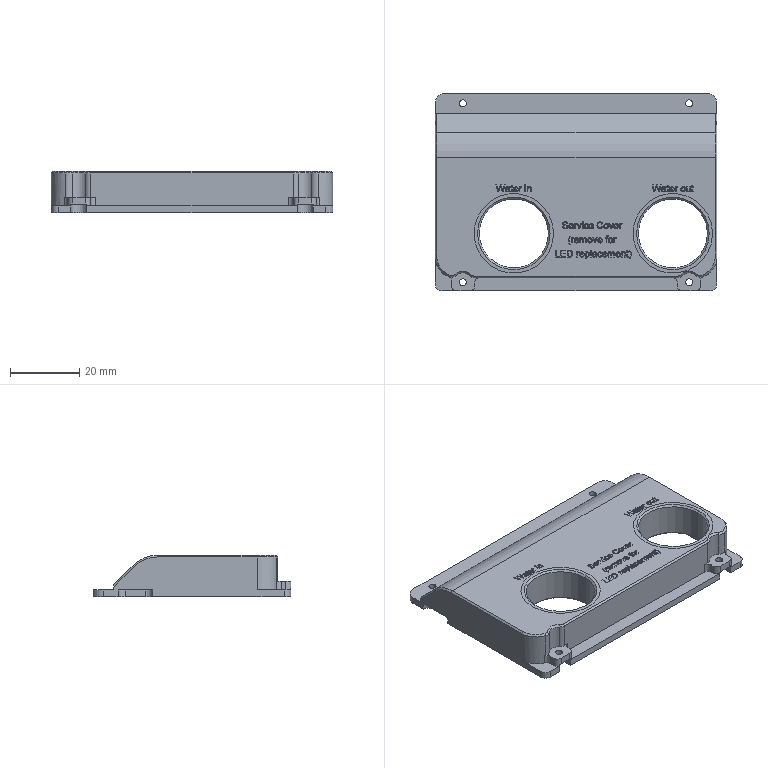NC program | NX | posted by the shop | part box 81.5 x 57.25 x 12.01 mm
Lines 1 to 947 of 2587:
%
G40 G17 G49 G80 G90
M05
M09
G91 G28 Z0.0
M01
T02 M06
S6500 M03
(ToolName=D8-25-D8-60-3T-Rough D.=8.00 R.=0.00)
 (0.15)(0.10)
G00 G90 G54 X-14.767 Y-10.373
G43 Z49.989 H02 M08
Z.5
G01 X-15.531 Y-9.312 Z.477 F3000.
X-16.643 Y-8.614 Z.454
X-17.93 Y-8.357 Z.431
X-19.224 Y-8.575 Z.409
X-20.357 Y-9.238 Z.386
X-21.179 Y-10.261 Z.363
X-21.584 Y-11.51 Z.34
X-21.518 Y-12.821 Z.317
X-20.991 Y-14.023 Z.294
X-20.07 Y-14.958 Z.272
X-18.877 Y-15.505 Z.249
X-17.568 Y-15.593 Z.226
X-16.313 Y-15.208 Z.203
X-15.276 Y-14.403 Z.18
X-14.594 Y-13.281 Z.157
X-14.356 Y-11.991 Z.134
X-14.591 Y-10.7 Z.112
X-15.271 Y-9.577 Z.089
X-16.306 Y-8.769 Z.066
X-17.56 Y-8.382 Z.043
X-18.87 Y-8.466 Z.02
X-20.064 Y-9.011 Z-.003
X-20.986 Y-9.944 Z-.025
X-21.517 Y-11.145 Z-.048
X-21.585 Y-12.456 Z-.071
X-21.183 Y-13.705 Z-.094
X-20.363 Y-14.73 Z-.117
X-19.232 Y-15.396 Z-.14
X-17.938 Y-15.616 Z-.163
X-16.65 Y-15.362 Z-.185
X-15.537 Y-14.667 Z-.208
X-14.744 Y-13.621 Z-.231
X-14.375 Y-12.361 Z-.254
X-14.478 Y-11.053 Z-.277
X-15.039 Y-9.866 Z-.3
X-15.986 Y-8.957 Z-.322
X-17.194 Y-8.444 Z-.345
X-18.506 Y-8.394 Z-.368
X-19.749 Y-8.814 Z-.391
X-20.762 Y-9.649 Z-.414
X-21.412 Y-10.789 Z-.437
X-21.614 Y-12.086 Z-.46
X-21.342 Y-13.37 Z-.482
X-20.63 Y-14.473 Z-.505
X-19.573 Y-15.251 Z-.528
X-18.309 Y-15.602 Z-.551
X-17.002 Y-15.481 Z-.574
X-15.823 Y-14.903 Z-.597
X-14.928 Y-13.943 Z-.62
X-14.432 Y-12.728 Z-.642
X-14.401 Y-11.415 Z-.665
X-14.838 Y-10.178 Z-.688
X-15.687 Y-9.177 Z-.711
X-16.837 Y-8.543 Z-.734
X-18.136 Y-8.36 Z-.757
X-19.416 Y-8.651 Z-.779
X-20.509 Y-9.378 Z-.802
X-21.272 Y-10.446 Z-.825
X-21.605 Y-11.715 Z-.848
X-21.465 Y-13.02 Z-.871
X-20.87 Y-14.19 Z-.894
X-19.898 Y-15.072 Z-.917
X-18.676 Y-15.55 Z-.939
X-17.363 Y-15.563 Z-.962
X-16.132 Y-15.108 Z-.985
X-15.143 Y-14.245 Z-1.008
X-14.526 Y-13.086 Z-1.031
X-14.361 Y-11.784 Z-1.054
X-14.67 Y-10.509 Z-1.076
X-15.412 Y-9.426 Z-1.099
X-16.491 Y-8.679 Z-1.122
X-17.765 Y-8.363 Z-1.145
X-19.068 Y-8.522 Z-1.168
X-20.23 Y-9.134 Z-1.191
X-21.098 Y-10.118 Z-1.214
X-21.559 Y-11.347 Z-1.236
X-21.553 Y-12.66 Z-1.259
X-21.08 Y-13.884 Z-1.282
X-20.203 Y-14.861 Z-1.305
X-19.036 Y-15.461 Z-1.328
X-17.731 Y-15.608 Z-1.351
X-16.46 Y-15.281 Z-1.373
X-15.389 Y-14.523 Z-1.396
X-14.656 Y-13.434 Z-1.419
X-14.359 Y-12.155 Z-1.442
X-14.537 Y-10.855 Z-1.465
X-15.165 Y-9.702 Z-1.488
X-16.162 Y-8.848 Z-1.511
X-17.397 Y-8.405 Z-1.533
X-18.709 Y-8.43 Z-1.556
X-19.927 Y-8.919 Z-1.579
X-20.891 Y-9.81 Z-1.602
X-21.475 Y-10.986 Z-1.625
X-21.603 Y-12.292 Z-1.648
X-21.258 Y-13.559 Z-1.67
X-20.485 Y-14.619 Z-1.693
X-19.385 Y-15.336 Z-1.716
X-18.102 Y-15.615 Z-1.739
X-16.804 Y-15.419 Z-1.762
X-15.661 Y-14.775 Z-1.785
X-14.821 Y-13.766 Z-1.808
X-14.396 Y-12.524 Z-1.83
X-14.439 Y-11.212 Z-1.853
X-14.946 Y-10.002 Z-1.876
X-15.851 Y-9.051 Z-1.899
X-17.034 Y-8.484 Z-1.922
X-18.342 Y-8.374 Z-1.945
X-19.604 Y-8.737 Z-1.967
X-20.654 Y-9.525 Z-1.99
X-21.354 Y-10.635 Z-2.013
X-21.615 Y-11.922 Z-2.036
X-21.401 Y-13.216 Z-2.059
X-20.74 Y-14.351 Z-2.082
X-19.719 Y-15.176 Z-2.105
X-18.472 Y-15.584 Z-2.127
X-17.161 Y-15.522 Z-2.15
X-15.958 Y-14.997 Z-2.173
X-15.019 Y-14.079 Z-2.196
X-14.469 Y-12.888 Z-2.219
X-14.379 Y-11.578 Z-2.242
X-14.76 Y-10.322 Z-2.265
X-15.562 Y-9.284 Z-2.287
X-16.682 Y-8.599 Z-2.31
X-17.972 Y-8.357 Z-2.333
X-19.264 Y-8.589 Z-2.356
X-20.388 Y-9.266 Z-2.379
X-21.199 Y-10.298 Z-2.402
X-21.589 Y-11.551 Z-2.424
X-21.509 Y-12.862 Z-2.447
X-20.967 Y-14.057 Z-2.47
X-20.036 Y-14.982 Z-2.493
X-18.837 Y-15.516 Z-2.516
X-17.526 Y-15.588 Z-2.539
X-16.275 Y-15.189 Z-2.562
X-15.249 Y-14.371 Z-2.584
X-14.579 Y-13.242 Z-2.607
X-14.356 Y-11.949 Z-2.63
X-14.607 Y-10.66 Z-2.653
X-15.299 Y-9.545 Z-2.676
X-16.343 Y-8.75 Z-2.699
X-17.602 Y-8.377 Z-2.721
X-18.91 Y-8.477 Z-2.744
X-20.098 Y-9.035 Z-2.767
X-21.01 Y-9.979 Z-2.79
X-21.526 Y-11.186 Z-2.813
X-21.579 Y-12.497 Z-2.836
X-21.163 Y-13.742 Z-2.859
X-20.331 Y-14.757 Z-2.881
X-19.192 Y-15.41 Z-2.904
X-17.896 Y-15.616 Z-2.927
X-16.611 Y-15.346 Z-2.95
X-15.506 Y-14.638 Z-2.973
X-14.725 Y-13.583 Z-2.996
X-14.371 Y-12.319 Z-3.018
X-14.489 Y-11.012 Z-3.041
X-15.064 Y-9.832 Z-3.064
X-16.021 Y-8.934 Z-3.087
X-17.235 Y-8.435 Z-3.11
X-18.547 Y-8.4 Z-3.133
X-19.786 Y-8.835 Z-3.156
X-20.789 Y-9.681 Z-3.178
X-21.426 Y-10.829 Z-3.201
X-21.613 Y-12.128 Z-3.224
X-21.325 Y-13.409 Z-3.247
X-20.601 Y-14.504 Z-3.27
X-19.535 Y-15.269 Z-3.293
X-18.267 Y-15.606 Z-3.315
X-16.961 Y-15.469 Z-3.338
X-15.79 Y-14.877 Z-3.361
X-14.905 Y-13.907 Z-3.384
X-14.424 Y-12.686 Z-3.407
X-14.408 Y-11.374 Z-3.43
X-14.859 Y-10.142 Z-3.453
X-15.72 Y-9.15 Z-3.475
X-16.877 Y-8.53 Z-3.498
X-18.178 Y-8.362 Z-3.521
X-19.455 Y-8.667 Z-3.544
X-20.539 Y-9.407 Z-3.567
X-21.29 Y-10.484 Z-3.59
X-21.608 Y-11.757 Z-3.612
X-21.453 Y-13.061 Z-3.635
X-20.844 Y-14.223 Z-3.658
X-19.862 Y-15.094 Z-3.681
X-18.634 Y-15.558 Z-3.704
X-17.322 Y-15.556 Z-3.727
X-16.096 Y-15.086 Z-3.75
X-15.117 Y-14.212 Z-3.772
X-14.514 Y-13.046 Z-3.795
X-14.364 Y-11.742 Z-3.818
X-14.687 Y-10.47 Z-3.841
X-15.442 Y-9.396 Z-3.864
X-16.53 Y-8.661 Z-3.887
X-17.808 Y-8.361 Z-3.909
X-19.109 Y-8.535 Z-3.932
X-20.263 Y-9.16 Z-3.955
X-21.119 Y-10.155 Z-3.978
X-21.566 Y-11.389 Z-4.001
X-21.545 Y-12.701 Z-4.024
X-21.058 Y-13.92 Z-4.047
X-20.169 Y-14.886 Z-4.069
X-18.995 Y-15.473 Z-4.092
X-17.689 Y-15.605 Z-4.115
X-16.422 Y-15.263 Z-4.138
X-15.359 Y-14.493 Z-4.161
X-14.64 Y-13.395 Z-4.184
X-14.358 Y-12.113 Z-4.207
X-14.55 Y-10.815 Z-4.229
X-15.191 Y-9.669 Z-4.252
X-16.198 Y-8.827 Z-4.275
X-17.438 Y-8.398 Z-4.298
X-18.75 Y-8.438 Z-4.321
X-19.962 Y-8.942 Z-4.344
X-20.916 Y-9.844 Z-4.366
X-21.486 Y-11.026 Z-4.389
X-21.599 Y-12.334 Z-4.412
X-21.239 Y-13.596 Z-4.435
X-20.454 Y-14.648 Z-4.458
X-19.346 Y-15.352 Z-4.481
X-18.06 Y-15.616 Z-4.504
X-16.765 Y-15.405 Z-4.526
X-15.629 Y-14.748 Z-4.549
X-14.801 Y-13.729 Z-4.572
X-14.39 Y-12.483 Z-4.595
X-14.448 Y-11.171 Z-4.618
X-14.969 Y-9.967 Z-4.641
X-15.885 Y-9.026 Z-4.663
X-17.075 Y-8.473 Z-4.686
X-18.384 Y-8.379 Z-4.709
X-19.641 Y-8.756 Z-4.732
X-20.682 Y-9.556 Z-4.755
X-21.37 Y-10.674 Z-4.778
X-21.615 Y-11.964 Z-4.801
X-21.386 Y-13.256 Z-4.823
X-20.713 Y-14.383 Z-4.846
X-19.682 Y-15.196 Z-4.869
X-18.43 Y-15.589 Z-4.892
X-17.12 Y-15.512 Z-4.915
X-15.923 Y-14.974 Z-4.938
X-14.995 Y-14.045 Z-4.96
X-14.459 Y-12.847 Z-4.983
X-14.384 Y-11.537 Z-5.006
X-14.779 Y-10.285 Z-5.029
X-15.594 Y-9.256 Z-5.052
X-16.721 Y-8.584 Z-5.075
X-18.014 Y-8.357 Z-5.098
X-19.303 Y-8.604 Z-5.12
X-20.42 Y-9.294 Z-5.143
X-21.218 Y-10.336 Z-5.166
X-21.594 Y-11.593 Z-5.189
X-21.498 Y-12.902 Z-5.212
X-20.943 Y-14.092 Z-5.235
X-20.001 Y-15.006 Z-5.257
X-18.796 Y-15.525 Z-5.28
X-17.484 Y-15.582 Z-5.303
X-16.238 Y-15.169 Z-5.326
X-15.221 Y-14.339 Z-5.349
X-14.565 Y-13.202 Z-5.372
X-14.356 Y-11.907 Z-5.395
X-14.622 Y-10.621 Z-5.417
X-15.328 Y-9.514 Z-5.44
X-16.381 Y-8.731 Z-5.463
X-17.644 Y-8.373 Z-5.486
X-18.951 Y-8.487 Z-5.509
X-20.132 Y-9.06 Z-5.532
X-21.033 Y-10.014 Z-5.554
X-21.535 Y-11.227 Z-5.577
X-21.573 Y-12.539 Z-5.6
X-21.142 Y-13.779 Z-5.623
X-20.298 Y-14.784 Z-5.646
X-19.152 Y-15.424 Z-5.669
X-17.854 Y-15.614 Z-5.692
X-16.572 Y-15.33 Z-5.714
X-15.476 Y-14.609 Z-5.737
X-14.707 Y-13.545 Z-5.76
X-14.367 Y-12.277 Z-5.783
X-14.5 Y-10.971 Z-5.806
X-15.089 Y-9.798 Z-5.829
X-16.057 Y-8.911 Z-5.851
X-17.277 Y-8.427 Z-5.874
X-18.589 Y-8.407 Z-5.897
X-19.822 Y-8.856 Z-5.92
X-20.816 Y-9.714 Z-5.943
X-21.439 Y-10.869 Z-5.966
X-21.611 Y-12.17 Z-5.989
X-21.309 Y-13.447 Z-6.011
X-20.572 Y-14.534 Z-6.034
X-19.497 Y-15.287 Z-6.057
X-18.225 Y-15.609 Z-6.08
X-16.921 Y-15.457 Z-6.103
X-15.756 Y-14.852 Z-6.126
X-14.883 Y-13.871 Z-6.149
X-14.416 Y-12.645 Z-6.171
X-14.415 Y-11.332 Z-6.194
X-14.881 Y-10.105 Z-6.217
X-15.753 Y-9.124 Z-6.24
X-16.917 Y-8.518 Z-6.263
X-18.221 Y-8.364 Z-6.286
X-19.493 Y-8.685 Z-6.308
X-20.569 Y-9.437 Z-6.331
X-21.307 Y-10.522 Z-6.354
X-21.611 Y-11.799 Z-6.377
X-21.44 Y-13.101 Z-6.4
X-20.818 Y-14.257 Z-6.423
X-19.826 Y-15.116 Z-6.446
X-18.593 Y-15.566 Z-6.468
X-17.28 Y-15.548 Z-6.491
X-16.06 Y-15.064 Z-6.514
X-15.092 Y-14.178 Z-6.537
X-14.501 Y-13.006 Z-6.56
X-14.367 Y-11.7 Z-6.583
X-14.705 Y-10.432 Z-6.605
X-15.473 Y-9.367 Z-6.628
X-16.568 Y-8.645 Z-6.651
X-17.85 Y-8.359 Z-6.674
X-19.149 Y-8.548 Z-6.697
X-20.295 Y-9.186 Z-6.72
X-21.14 Y-10.191 Z-6.743
X-21.573 Y-11.43 Z-6.765
X-21.536 Y-12.742 Z-6.788
X-21.035 Y-13.956 Z-6.811
X-20.136 Y-14.911 Z-6.834
X-18.955 Y-15.485 Z-6.857
X-17.648 Y-15.601 Z-6.88
X-16.384 Y-15.244 Z-6.902
X-15.33 Y-14.462 Z-6.925
X-14.624 Y-13.356 Z-6.948
X-14.356 Y-12.071 Z-6.971
X-14.564 Y-10.775 Z-6.994
X-15.218 Y-9.637 Z-7.017
X-16.235 Y-8.807 Z-7.04
X-17.48 Y-8.392 Z-7.062
X-18.792 Y-8.447 Z-7.085
X-19.998 Y-8.965 Z-7.108
X-20.941 Y-9.878 Z-7.131
X-21.497 Y-11.067 Z-7.154
X-21.595 Y-12.376 Z-7.177
X-21.22 Y-13.634 Z-7.199
X-20.423 Y-14.677 Z-7.222
X-19.307 Y-15.368 Z-7.245
X-18.018 Y-15.617 Z-7.268
X-16.725 Y-15.391 Z-7.291
X-15.597 Y-14.72 Z-7.314
X-14.781 Y-13.692 Z-7.337
X-14.384 Y-12.441 Z-7.359
X-14.458 Y-11.13 Z-7.382
X-14.993 Y-9.932 Z-7.405
X-15.919 Y-9.002 Z-7.428
X-17.116 Y-8.462 Z-7.451
X-18.426 Y-8.384 Z-7.474
X-19.679 Y-8.776 Z-7.496
X-20.71 Y-9.588 Z-7.519
X-21.385 Y-10.714 Z-7.542
X-21.615 Y-12.006 Z-7.565
X-21.371 Y-13.295 Z-7.588
X-20.685 Y-14.414 Z-7.611
X-19.645 Y-15.215 Z-7.634
X-18.388 Y-15.594 Z-7.656
X-17.079 Y-15.502 Z-7.679
X-15.888 Y-14.95 Z-7.702
X-14.972 Y-14.01 Z-7.725
X-14.449 Y-12.806 Z-7.748
X-14.389 Y-11.495 Z-7.771
X-14.799 Y-10.248 Z-7.793
X-15.626 Y-9.228 Z-7.816
X-16.761 Y-8.57 Z-7.839
X-18.056 Y-8.357 Z-7.862
X-19.342 Y-8.62 Z-7.885
X-20.451 Y-9.322 Z-7.908
X-21.237 Y-10.373 Z-7.931
X-21.598 Y-11.635 Z-7.953
X-21.487 Y-12.943 Z-7.976
X-20.918 Y-14.126 Z-7.999
X-19.966 Y-15.029 Z-8.022
X-18.754 Y-15.534 Z-8.045
X-17.442 Y-15.576 Z-8.068
X-16.202 Y-15.148 Z-8.091
X-15.194 Y-14.307 Z-8.113
X-14.551 Y-13.163 Z-8.136
X-14.358 Y-11.864 Z-8.159
X-14.638 Y-10.582 Z-8.182
X-15.357 Y-9.484 Z-8.205
X-16.419 Y-8.712 Z-8.228
X-17.685 Y-8.369 Z-8.25
X-18.992 Y-8.499 Z-8.273
X-20.166 Y-9.085 Z-8.296
X-21.056 Y-10.05 Z-8.319
X-21.544 Y-11.268 Z-8.342
X-21.567 Y-12.581 Z-8.365
X-21.121 Y-13.815 Z-8.388
X-20.266 Y-14.811 Z-8.41
X-19.112 Y-15.437 Z-8.433
X-17.812 Y-15.613 Z-8.456
X-16.533 Y-15.314 Z-8.479
X-15.445 Y-14.58 Z-8.502
X-14.689 Y-13.507 Z-8.525
X-14.364 Y-12.235 Z-8.547
X-14.512 Y-10.931 Z-8.57
X-15.115 Y-9.765 Z-8.593
X-16.093 Y-8.889 Z-8.616
X-17.318 Y-8.419 Z-8.639
X-18.63 Y-8.414 Z-8.662
X-19.859 Y-8.877 Z-8.685
X-20.842 Y-9.747 Z-8.707
X-21.452 Y-10.909 Z-8.73
X-21.608 Y-12.212 Z-8.753
X-21.291 Y-13.486 Z-8.776
X-20.542 Y-14.564 Z-8.799
X-19.459 Y-15.304 Z-8.822
X-18.182 Y-15.611 Z-8.844
X-16.881 Y-15.444 Z-8.867
X-15.723 Y-14.825 Z-8.89
X-14.861 Y-13.835 Z-8.913
X-14.408 Y-12.604 Z-8.936
X-14.423 Y-11.291 Z-8.959
X-14.903 Y-10.07 Z-8.982
X-15.786 Y-9.099 Z-9.004
X-16.957 Y-8.505 Z-9.027
X-18.263 Y-8.367 Z-9.05
X-19.532 Y-8.702 Z-9.073
X-20.598 Y-9.467 Z-9.096
X-21.324 Y-10.561 Z-9.119
X-21.613 Y-11.841 Z-9.141
X-21.427 Y-13.141 Z-9.164
X-20.792 Y-14.289 Z-9.187
X-19.789 Y-15.137 Z-9.21
X-18.551 Y-15.572 Z-9.233
X-17.239 Y-15.539 Z-9.256
X-16.025 Y-15.042 Z-9.279
X-15.066 Y-14.144 Z-9.301
X-14.49 Y-12.965 Z-9.324
X-14.37 Y-11.658 Z-9.347
X-14.724 Y-10.394 Z-9.37
X-15.503 Y-9.338 Z-9.393
X-16.607 Y-8.628 Z-9.416
X-17.892 Y-8.358 Z-9.438
X-19.188 Y-8.562 Z-9.461
X-20.328 Y-9.213 Z-9.484
X-21.161 Y-10.228 Z-9.507
X-21.579 Y-11.472 Z-9.53
X-21.527 Y-12.783 Z-9.553
X-21.012 Y-13.991 Z-9.576
X-20.102 Y-14.936 Z-9.598
X-18.914 Y-15.496 Z-9.621
X-17.606 Y-15.597 Z-9.644
X-16.347 Y-15.226 Z-9.667
X-15.302 Y-14.431 Z-9.69
X-14.608 Y-13.317 Z-9.713
X-14.356 Y-12.029 Z-9.736
X-14.578 Y-10.735 Z-9.758
X-15.246 Y-9.605 Z-9.781
X-16.272 Y-8.787 Z-9.804
X-17.522 Y-8.386 Z-9.827
X-18.833 Y-8.457 Z-9.85
X-20.032 Y-8.989 Z-9.873
X-20.965 Y-9.913 Z-9.895
X-21.508 Y-11.108 Z-9.918
X-21.59 Y-12.418 Z-9.941
X-21.201 Y-13.672 Z-9.964
X-20.391 Y-14.705 Z-9.987
X-19.268 Y-15.383 Z-10.01
X-17.976 Y-15.617 Z-10.033
X-16.686 Y-15.376 Z-10.055
X-15.565 Y-14.692 Z-10.078
X-14.761 Y-13.655 Z-10.101
X-14.379 Y-12.399 Z-10.124
X-14.468 Y-11.089 Z-10.147
X-15.017 Y-9.897 Z-10.17
X-15.954 Y-8.978 Z-10.192
X-17.157 Y-8.453 Z-10.215
X-18.468 Y-8.389 Z-10.238
X-19.716 Y-8.796 Z-10.261
X-20.738 Y-9.62 Z-10.284
X-21.399 Y-10.753 Z-10.307
X-21.615 Y-12.048 Z-10.33
X-21.356 Y-13.335 Z-10.352
X-20.656 Y-14.445 Z-10.375
X-19.607 Y-15.234 Z-10.398
X-18.346 Y-15.599 Z-10.421
X-17.038 Y-15.491 Z-10.444
X-15.854 Y-14.925 Z-10.467
X-14.948 Y-13.975 Z-10.489
X-14.44 Y-12.765 Z-10.512
X-14.395 Y-11.453 Z-10.535
X-14.819 Y-10.211 Z-10.558
X-15.658 Y-9.201 Z-10.581
X-16.801 Y-8.556 Z-10.604
X-18.098 Y-8.358 Z-10.627
X-19.381 Y-8.636 Z-10.649
X-20.482 Y-9.351 Z-10.672
X-21.256 Y-10.411 Z-10.695
X-21.602 Y-11.677 Z-10.718
X-21.476 Y-12.984 Z-10.741
X-20.893 Y-14.16 Z-10.764
X-19.93 Y-15.052 Z-10.786
X-18.713 Y-15.543 Z-10.809
X-17.401 Y-15.569 Z-10.832
X-16.165 Y-15.127 Z-10.855
X-15.167 Y-14.274 Z-10.878
X-14.538 Y-13.123 Z-10.901
X-14.359 Y-11.822 Z-10.924
X-14.655 Y-10.543 Z-10.946
X-15.386 Y-9.453 Z-10.969
X-16.457 Y-8.694 Z-10.992
X-17.727 Y-8.366 Z-11.015
X-19.032 Y-8.511 Z-11.038
X-20.2 Y-9.11 Z-11.061
X-21.078 Y-10.086 Z-11.083
X-21.552 Y-11.31 Z-11.106
X-21.559 Y-12.622 Z-11.129
X-21.1 Y-13.852 Z-11.152
X-20.233 Y-14.837 Z-11.175
X-19.072 Y-15.45 Z-11.198
X-17.77 Y-15.61 Z-11.221
X-16.495 Y-15.297 Z-11.243
X-15.415 Y-14.55 Z-11.266
X-14.672 Y-13.469 Z-11.289
X-14.361 Y-12.193 Z-11.312
X-14.525 Y-10.891 Z-11.335
X-15.141 Y-9.732 Z-11.358
X-16.129 Y-8.868 Z-11.38
X-17.359 Y-8.411 Z-11.403
X-18.672 Y-8.422 Z-11.426
X-19.895 Y-8.899 Z-11.449
X-20.868 Y-9.78 Z-11.472
X-21.464 Y-10.949 Z-11.495
X-21.606 Y-12.254 Z-11.518
X-21.274 Y-13.524 Z-11.54
X-20.512 Y-14.593 Z-11.563
X-19.42 Y-15.321 Z-11.586
X-18.14 Y-15.613 Z-11.609
X-16.841 Y-15.431 Z-11.632
X-15.69 Y-14.799 Z-11.655
X-14.84 Y-13.799 Z-11.678
X-14.401 Y-12.562 Z-11.7
X-14.431 Y-11.25 Z-11.723
X-14.926 Y-10.034 Z-11.746
X-15.82 Y-9.073 Z-11.769
X-16.998 Y-8.494 Z-11.792
X-18.305 Y-8.371 Z-11.815
X-19.57 Y-8.721 Z-11.837
X-20.628 Y-9.497 Z-11.86
X-21.34 Y-10.6 Z-11.883
X-21.614 Y-11.883 Z-11.906
X-21.414 Y-13.181 Z-11.929
X-20.765 Y-14.322 Z-11.952
X-19.753 Y-15.157 Z-11.975
X-18.51 Y-15.579 Z-11.997
X-17.198 Y-15.53 Z-12.02
X-15.989 Y-15.019 Z-12.043
X-15.042 Y-14.11 Z-12.066
X-14.479 Y-12.925 Z-12.089
X-14.374 Y-11.616 Z-12.112
X-14.742 Y-10.356 Z-12.134
X-15.534 Y-9.31 Z-12.157
X-16.646 Y-8.613 Z-12.18
X-17.934 Y-8.357 Z-12.203
X-19.228 Y-8.576 Z-12.226
X-20.36 Y-9.241 Z-12.249
X-21.181 Y-10.265 Z-12.272
X-21.585 Y-11.514 Z-12.294
X-21.517 Y-12.825 Z-12.317
X-20.989 Y-14.026 Z-12.34
X-20.067 Y-14.961 Z-12.363
X-18.873 Y-15.506 Z-12.386
X-17.564 Y-15.592 Z-12.409
X-16.309 Y-15.206 Z-12.431
X-15.274 Y-14.4 Z-12.454
X-14.593 Y-13.278 Z-12.477
X-14.386 Y-11.987 Z-12.5
G03 X-18.366 Y-15.603 I-3.618 J-.017
X-14.817 Y-13.831 I.355 J3.728
X-18.276 Y-8.002 I-3.129 J2.085
X-15.206 Y-14.915 I.302 J-4.004
X-18.949 Y-7.697 I-2.774 J3.14
X-15.204 Y-15.455 I.979 J-4.31
X-18.818 Y-7.244 I-2.783 J3.676
X-15.366 Y-16.09 I.848 J-4.766
X-18.76 Y-6.792 I-2.628 J4.309
X-15.958 Y-16.89 I.782 J-5.221
X-19.052 Y-6.379 I-2.046 J5.109
X-15.814 Y-17.33 I1.078 J-5.636
X-18.67 Y-5.852 I-2.183 J5.551
X-16.332 Y-18.002 I.693 J-6.167
X-18.383 Y-5.343 I-1.664 J6.226
X-16.782 Y-18.601 I.403 J-6.677
X-12.164 Y-15.539 I-1.188 J6.806
X-11.144 Y-11.897 I-5.795 J3.587
X-12.188 Y-8.35 I-7.258 J-.21
X-14.923 Y-5.866 I-6.084 J-3.949
X-18.582 Y-5.168 I-3.141 J-6.526
X-21.985 Y-6.432 I.767 J-7.278
X-24.383 Y-9.553 I4.293 J-5.779
X-24.83 Y-12.051 I7.259 J-2.588
X-23.801 Y-15.595 I7.257 J.186
X-20.097 Y-18.495 I5.962 J3.798
X-16.54 Y-18.674 I2.129 J6.875
X-12.564 Y-16.161 I-1.577 J6.896
X-11.897 Y-15.092 I-6.413 J4.745
X-12.439 Y-13.982 I-.739 J.326
G01 X-13.445 Y-13.729
X-13.47 Y-13.723 Z-12.499
X-13.494 Y-13.717 Z-12.497
X-13.518 Y-13.711 Z-12.494
X-13.542 Y-13.704 Z-12.49
X-13.567 Y-13.698 Z-12.484
X-13.591 Y-13.692 Z-12.477
X-13.615 Y-13.686 Z-12.468
X-13.639 Y-13.68 Z-12.458
X-13.664 Y-13.674 Z-12.447
X-13.688 Y-13.668 Z-12.433
X-13.712 Y-13.662 Z-12.418
X-13.736 Y-13.656 Z-12.4
X-13.761 Y-13.65 Z-12.38
X-13.785 Y-13.643 Z-12.357
X-13.809 Y-13.637 Z-12.331
X-13.833 Y-13.631 Z-12.3
X-13.858 Y-13.625 Z-12.263
X-13.882 Y-13.619 Z-12.218
X-13.906 Y-13.613 Z-12.156
X-13.93 Y-13.607 Z-12.
G00 Z49.989
X-49.561 Y.83
Z-12.
G01 X-49.536 Y.832 Z-12.156
X-49.511 Y.833 Z-12.218
X-49.486 Y.834 Z-12.263
X-49.461 Y.835 Z-12.3
X-49.436 Y.836 Z-12.331
X-49.411 Y.837 Z-12.357
X-49.386 Y.839 Z-12.38
X-49.362 Y.84 Z-12.4
X-49.337 Y.841 Z-12.418
X-49.312 Y.842 Z-12.433
X-49.287 Y.843 Z-12.447
X-49.262 Y.845 Z-12.458
X-49.237 Y.846 Z-12.468
X-49.212 Y.847 Z-12.477
X-49.187 Y.848 Z-12.484
X-49.162 Y.849 Z-12.49
X-49.137 Y.851 Z-12.494
X-49.112 Y.852 Z-12.497
X-49.087 Y.853 Z-12.499
X-49.062 Y.854 Z-12.5
X-47.756 Y.917
G03 X-47.058 Y1.391 I-.039 J.808
X-46.412 Y4.246 I-7.771 J3.259
X-46.209 Y11.329 I-90.833 J6.149
G01 X-46.199 Y18.995
X-46.187 Y28.955
G02 X-44.34 Y32.064 I4.509 J-.575
X-40.442 Y33.686 I5.341 J-7.341
X-34.827 Y34.146 I5.601 J-33.883
X-24.148 Y34.198 I8.788 J-707.178
G01 X40.702
G02 X43.826 Y32.627 I-.212 J-4.312
X45.598 Y28.862 I-6.451 J-5.336
X46.131 Y23.437 I-28.551 J-5.542
X46.198 Y11.437 I-611.378 J-9.43
G01 X46.197 Y-28.752
G02 X44.564 Y-31.907 I-4.343 J.248
X40.839 Y-33.616 I-5.263 J6.557
X35.532 Y-34.13 I-5.476 J28.892
X23.532 Y-34.198 I-9.449 J603.833
G01 X-40.819 Y-34.196
G02 X-43.95 Y-32.513 I.337 J4.382
X-45.654 Y-28.656 I6.796 J5.308
X-46.142 Y-23.045 I32.128 J5.619
X-46.198 Y-12.845 I683.633 J8.815
X-46.18 Y-.925 I885.538 J4.687
X-45.716 Y3.51 I189.462 J-17.597
G03 X-45.413 Y12.592 I-109.599 J8.197
G01 X-45.399 Y20.256
G02 X-45.379 Y26.735 I305.297 J2.269
X-42.688 Y31.159 I5.98 J-.607
X-38.179 Y32.868 I6.15 J-9.425
X-31.783 Y33.346 I6.354 J-41.918
X-20.023 Y33.398 I9.161 J-747.573
G01 X38.315
G02 X43.013 Y30.89 I-.134 J-5.906
X44.259 Y28.519 I-7.486 J-5.45
G01 X44.469 Y28.069
G02 X45.184 Y23.832 I-17.534 J-5.135
X45.392 Y14.597 I-140.468 J-7.785
G01 X45.397 Y8.237
Y-26.352
G02 X43.383 Y-30.627 I-5.773 J.108
G01 X43.098 Y-30.975
X42.165 Y-31.739
X41.102 Y-32.307
G02 X36.866 Y-33.128 I-5.347 J16.25
X29.312 Y-33.382 I-6.965 J94.941
G01 X20.552 Y-33.398
X-38.412 Y-33.397
G02 X-42.704 Y-31.297 I.177 J5.799
G01 X-43.1 Y-30.973
X-43.864 Y-30.04
X-44.432 Y-28.977
G02 X-45.054 Y-25.984 I11.124 J3.871
X-45.373 Y-18.554 I76.758 J7.023
G01 X-45.397 Y-8.594
X-45.393 Y22.274
G03 X-44.95 Y23.926 I-10.543 J3.713
G01 X-44.9 Y24.267
G02 X-44.791 Y26.868 I16. J.633
G01 X-44.468 Y28.072
X-43.941 Y29.201
X-43.226 Y30.222
X-42.345 Y31.103
X-41.324 Y31.818
X-40.194 Y32.344
X-38.99 Y32.666
X-37.749 Y32.775
X37.751
X38.993 Y32.666
X40.197 Y32.343
X41.326 Y31.816
X42.347 Y31.101
X43.228 Y30.22
X43.943 Y29.199
X44.469 Y28.069
X44.791 Y26.865
X44.9 Y25.624
Y-26.626
X44.781 Y-27.826
X44.431 Y-28.98
X43.863 Y-30.043
X43.098 Y-30.975
X42.165 Y-31.739
X41.102 Y-32.307
X39.948 Y-32.657
X38.749 Y-32.775
X30.566 Y-32.774
X-34.673 Y-32.771
X-38.751 Y-32.775
X-39.951 Y-32.656
X-41.105 Y-32.306
X-42.168 Y-31.738
X-43.1 Y-30.973
X-43.864 Y-30.04
X-44.432 Y-28.977
X-44.782 Y-27.823
X-44.9 Y-26.625
Y24.315
G03 X-45.734 Y25.123 I-.808 J0.0
G01 X-46.865 Y25.085
X-46.89 Z-12.499
X-46.915 Y25.084 Z-12.497
X-46.94 Y25.083 Z-12.494
X-46.965 Y25.082 Z-12.49
X-46.99 Y25.081 Z-12.484
X-47.015 Z-12.477
X-47.039 Y25.08 Z-12.468
X-47.064 Y25.079 Z-12.458
X-47.089 Y25.078 Z-12.447
X-47.114 Y25.077 Z-12.433
X-47.139 Y25.076 Z-12.418
X-47.164 Z-12.4
X-47.189 Y25.075 Z-12.38
X-47.214 Y25.074 Z-12.357
X-47.239 Y25.073 Z-12.331
X-47.264 Y25.072 Z-12.3
X-47.289 Z-12.263
X-47.314 Y25.071 Z-12.218
X-47.339 Y25.07 Z-12.156
X-47.364 Y25.069 Z-12.
G00 Z49.989
X-33.296 Y-35.238
Z-9.41
G01 X-33.294 Y-35.213 Z-9.566
X-33.292 Y-35.188 Z-9.627
X-33.29 Y-35.163 Z-9.673
X-33.288 Y-35.138 Z-9.71
X-33.286 Y-35.113 Z-9.74
X-33.283 Y-35.088 Z-9.767
X-33.281 Y-35.063 Z-9.79
X-33.279 Y-35.039 Z-9.81
X-33.277 Y-35.014 Z-9.827
X-33.275 Y-34.989 Z-9.843
X-33.272 Y-34.964 Z-9.856
X-33.27 Y-34.939 Z-9.868
X-33.268 Y-34.914 Z-9.878
X-33.266 Y-34.889 Z-9.887
X-33.264 Y-34.864 Z-9.894
X-33.262 Y-34.839 Z-9.899
X-33.259 Y-34.814 Z-9.904
X-33.257 Y-34.789 Z-9.907
X-33.255 Y-34.765 Z-9.909
X-33.253 Y-34.74 Z-9.91
X-33.158 Y-33.654
G03 X-33.963 Y-32.775 I-.805 J.07
G02 X-36.428 Y-32.433 I-.263 J7.166
X-38.932 Y-31.912 I4.125 J26.106
X-43.049 Y-27.94 I1.816 J6.002
X-43.916 Y-23.419 I15.199 J5.259
G03 X-44.018 Y-22.963 I-1.39 J-.073
G02 X-44.801 Y-20.24 I10.892 J4.604
G01 X-44.855 Y-19.462
X-44.801 Y-20.24
G03 X-43.994 Y-23.008 I11.473 J1.843
G02 X-43.457 Y-24.665 I-6.996 J-3.183
G03 X-42.347 Y-27.886 I13.047 J2.693
X-38.719 Y-31.002 I6.239 J3.595
G02 X-38.231 Y-31.323 I-.382 J-1.112
G03 X-36.123 Y-32.512 I3.998 J4.626
G02 X-38.311 Y-31.237 I1.719 J5.464
X-40.204 Y-29.158 I26.432 J25.97
X-41.979 Y-25.946 I11.318 J8.35
G03 X-42.514 Y-25.363 I-6.212 J-5.16
G01 X-43.35 Y-24.216
X-43.943 Y-23.104
G03 X-41.843 Y-26.065 I9.209 J4.305
G01 X-39.892 Y-28.694
X-39.461 Y-29.735
X-38.917 Y-30.584
G02 X-39.845 Y-28.802 I5.289 J3.887
G03 X-40.454 Y-27.233 I-4.182 J-.72
G01 X-41.526 Y-26.382
X-41.943 Y-25.952
X-41.526 Y-26.382
G02 X-40.297 Y-27.366 I-11.793 J-15.988
X-40.046 Y-27.869 I-.961 J-.793
G01 X-39.92 Y-28.456
G02 X-40.374 Y-29.361 I-.79 J-.17
G01 X-41.523 Y-29.886
X-41.546 Y-29.897 Z-9.909
X-41.569 Y-29.907 Z-9.907
X-41.592 Y-29.917 Z-9.904
X-41.614 Y-29.928 Z-9.899
X-41.637 Y-29.938 Z-9.894
X-41.66 Y-29.949 Z-9.887
X-41.683 Y-29.959 Z-9.878
X-41.705 Y-29.969 Z-9.868
X-41.728 Y-29.98 Z-9.856
X-41.751 Y-29.99 Z-9.843
X-41.774 Y-30. Z-9.827
X-41.796 Y-30.011 Z-9.81
X-41.819 Y-30.021 Z-9.79
X-41.842 Y-30.032 Z-9.767
X-41.865 Y-30.042 Z-9.74
X-41.887 Y-30.052 Z-9.71
X-41.91 Y-30.063 Z-9.673
X-41.933 Y-30.073 Z-9.627
X-41.956 Y-30.084 Z-9.566
X-41.978 Y-30.094 Z-9.41
G00 Z49.989
X-47.36 Y22.018
Z-9.41
G01 X-47.335 Y22.022 Z-9.566
X-47.311 Y22.025 Z-9.627
X-47.286 Y22.028 Z-9.673
X-47.261 Y22.031 Z-9.71
X-47.236 Y22.035 Z-9.74
X-47.211 Y22.038 Z-9.767
X-47.187 Y22.041 Z-9.79
X-47.162 Y22.045 Z-9.81
X-47.137 Y22.048 Z-9.827
X-47.112 Y22.051 Z-9.843
X-47.088 Y22.055 Z-9.856
X-47.063 Y22.058 Z-9.868
X-47.038 Y22.061 Z-9.878
X-47.013 Y22.065 Z-9.887
X-46.988 Y22.068 Z-9.894
X-46.964 Y22.071 Z-9.899
X-46.939 Y22.075 Z-9.904
X-46.914 Y22.078 Z-9.907
X-46.889 Y22.081 Z-9.909
X-46.865 Y22.085 Z-9.91
X-45.557 Y22.26
G03 X-44.861 Y22.97 I-.108 J.801
G02 X-44.62 Y24.078 I3.34 J-.146
X-43.776 Y26.983 I18.418 J-3.779
X-39.022 Y31.144 I6.607 J-2.754
X-34.285 Y31.846 I5.308 J-19.478
X-24.207 Y31.974 I7.905 J-225.893
G01 X35.473 Y31.975
G02 X39.407 Y31.307 I.373 J-9.728
X43.16 Y27.084 I-2.709 J-6.187
G03 X43.561 Y25.703 I70.953 J19.837
X43.995 Y25.212 I1.974 J1.307
G01 X44.489 Y24.426
X44.796 Y23.548
X44.863 Y22.952
X44.796 Y23.548
X44.489 Y24.426
X43.995 Y25.212
G02 X43.23 Y26.202 I1.829 J2.203
G03 X41.291 Y28.997 I-9.431 J-4.473
X36.975 Y31.085 I-5.603 J-6.078
X31.835 Y31.465 I-4.885 J-31.107
G01 X24.935 Y31.494
X-25.265 Y31.493
G03 X-34.442 Y31.326 I-1.812 J-152.805
X-38.738 Y30.548 I.659 J-15.9
X-43.022 Y26.541 I2.674 J-7.151
G02 X-43.404 Y25.803 I-4.189 J1.704
G01 X-43.995 Y25.212
X-44.489 Y24.426
X-44.667 Y23.916
X-44.489 Y24.426
X-43.995 Y25.212
G02 X-42.7 Y26.441 I23.763 J-23.762
X-38.756 Y29.264 I8.567 J-7.799
X-33.504 Y30.429 I6.454 J-16.684
X-24.991 Y30.686 I7.388 J-103.408
G01 X-18.811 Y30.694
X26.889 Y30.692
G02 X34.265 Y30.528 I1.454 J-100.36
X38.368 Y29.487 I-.546 J-10.755
X41.192 Y27.144 I-4.654 J-8.484
G03 X41.746 Y26.646 I1.312 J.899
G01 X42.551 Y26.364
X43.337 Y25.87
X43.634 Y25.573
X43.337 Y25.87
X42.551 Y26.364
G02 X41.468 Y26.769 I2.024 J7.056
G03 X39.3 Y28.256 I-55.759 J-78.987
X34.197 Y29.898 I-6.395 J-11.119
X28.088 Y30.197 I-5.692 J-53.89
G01 X21.668 Y30.214
X-21.812 Y30.212
G03 X-31.769 Y30.048 I-1.884 J-187.52
X-37.147 Y29.184 I.838 J-22.398
X-41.408 Y26.789 I3.99 J-12.087
G02 X-42.551 Y26.364 I-3.322 J7.187
G01 X-43.313 Y25.885
X-42.551 Y26.364
G02 X-41.138 Y26.783 I3.013 J-7.577
G01 X-38.025 Y27.957
G02 X-30.955 Y29.21 I8.291 J-26.21
X-21.179 Y29.41 I8.309 J-167.743
G01 X-15.899 Y29.413
X23.981 Y29.412